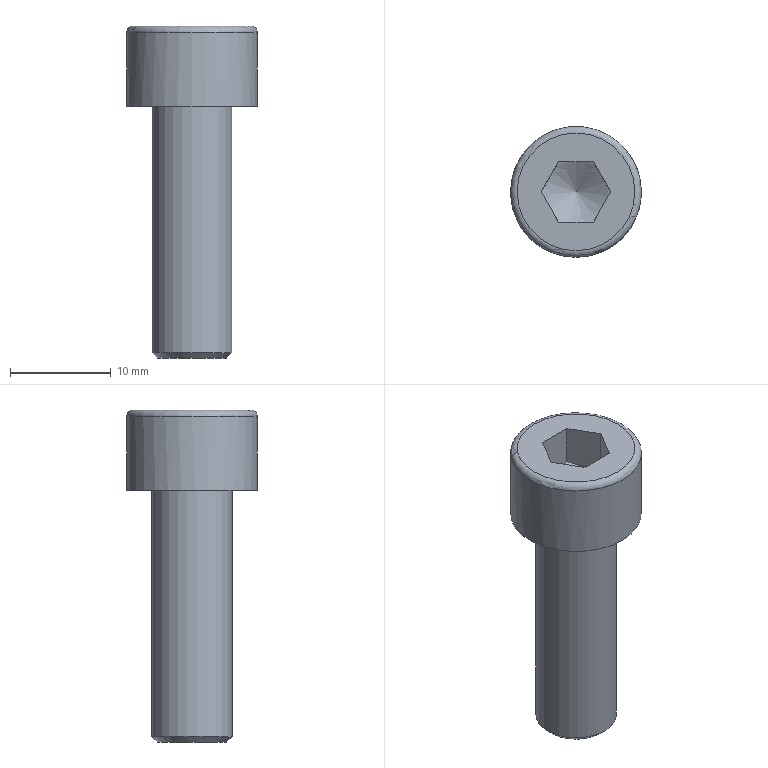Part | STEP file | 1_36 | 1 solid | 14 faces | box 13 x 13 x 33 mm | volume 2162 mm3 | plane 9 | cylinder 2 | cone 2 | torus 1 | commonest cylinder face diameters 8 x1 13 x1
STEP:
#1=CARTESIAN_POINT('',(0.,0.,0.));
#2=DIRECTION('',(0.,0.,1.));
#3=DIRECTION('',(1.,0.,0.));
#4=AXIS2_PLACEMENT_3D('',#1,#2,#3);
#5=CARTESIAN_POINT('',(0.,-6.5,-0.000000001));
#6=VERTEX_POINT('',#5);
#7=CARTESIAN_POINT('',(0.,0.,-0.000000001));
#8=DIRECTION('',(0.,0.,1.));
#9=DIRECTION('',(1.,0.,0.));
#10=AXIS2_PLACEMENT_3D('',#7,#8,#9);
#11=CIRCLE('',#10,6.5);
#12=CARTESIAN_POINT('',(0.,0.,3.675));
#13=DIRECTION('',(0.,0.,1.));
#14=DIRECTION('',(0.,-1.,0.));
#15=AXIS2_PLACEMENT_3D('',#12,#13,#14);
#16=CYLINDRICAL_SURFACE('',#15,6.5);
#17=CARTESIAN_POINT('',(-4.712,-3.675));
#18=DIRECTION('',(1.,0.));
#19=VECTOR('',#18,1.);
#20=LINE('',#17,#19);
#21=(GEOMETRIC_REPRESENTATION_CONTEXT(2)PARAMETRIC_REPRESENTATION_CONTEXT()REPRESENTATION_CONTEXT('',''));
#22=DEFINITIONAL_REPRESENTATION('',(#20),#21);
#23=PCURVE('',#16,#22);
#24=CARTESIAN_POINT('',(0.,3.25,0.));
#25=DIRECTION('',(0.,0.,-1.));
#26=DIRECTION('',(-1.,0.,0.));
#27=AXIS2_PLACEMENT_3D('',#24,#25,#26);
#28=PLANE('',#27);
#29=CARTESIAN_POINT('',(-6.5,-3.25));
#30=CARTESIAN_POINT('',(-6.5,8.008));
#31=CARTESIAN_POINT('',(3.25,2.379));
#32=CARTESIAN_POINT('',(13.,-3.25));
#33=CARTESIAN_POINT('',(3.25,-8.879));
#34=CARTESIAN_POINT('',(-6.5,-14.508));
#35=CARTESIAN_POINT('',(-6.5,-3.25));
#36=(BOUNDED_CURVE()B_SPLINE_CURVE(2,(#29,#30,#31,#32,#33,#34,#35),.UNSPECIFIED.,.T.,.F.)B_SPLINE_CURVE_WITH_KNOTS((1,2,2,2,2,1),(-2.094,0.,2.094,4.189,6.283,8.378),.UNSPECIFIED.)CURVE()GEOMETRIC_REPRESENTATION_ITEM()RATIONAL_B_SPLINE_CURVE((1.,0.5,1.,0.5,1.,0.5,1.))REPRESENTATION_ITEM(''));
#37=(GEOMETRIC_REPRESENTATION_CONTEXT(2)PARAMETRIC_REPRESENTATION_CONTEXT()REPRESENTATION_CONTEXT('',''));
#38=DEFINITIONAL_REPRESENTATION('',(#36),#37);
#39=PCURVE('',#28,#38);
#40=SURFACE_CURVE('',#11,(#23,#39),.PCURVE_S1.);
#41=EDGE_CURVE('',#6,#6,#40,.T.);
#42=ORIENTED_EDGE('',*,*,#41,.T.);
#43=CARTESIAN_POINT('',(0.,-6.5,7.35));
#44=VERTEX_POINT('',#43);
#45=CARTESIAN_POINT('',(0.,-6.5,-0.000000001));
#46=CARTESIAN_POINT('',(0.,-6.5,7.35));
#47=B_SPLINE_CURVE_WITH_KNOTS('',1,(#45,#46),.UNSPECIFIED.,.F.,.F.,(2,2),(-3.675,3.675),.PIECEWISE_BEZIER_KNOTS.);
#48=CARTESIAN_POINT('',(6.283,0.));
#49=DIRECTION('',(0.,1.));
#50=VECTOR('',#49,1.);
#51=LINE('',#48,#50);
#52=(GEOMETRIC_REPRESENTATION_CONTEXT(2)PARAMETRIC_REPRESENTATION_CONTEXT()REPRESENTATION_CONTEXT('',''));
#53=DEFINITIONAL_REPRESENTATION('',(#51),#52);
#54=PCURVE('',#16,#53);
#55=CARTESIAN_POINT('',(0.,0.));
#56=DIRECTION('',(0.,1.));
#57=VECTOR('',#56,1.);
#58=LINE('',#55,#57);
#59=(GEOMETRIC_REPRESENTATION_CONTEXT(2)PARAMETRIC_REPRESENTATION_CONTEXT()REPRESENTATION_CONTEXT('',''));
#60=DEFINITIONAL_REPRESENTATION('',(#58),#59);
#61=PCURVE('',#16,#60);
#62=SEAM_CURVE('',#47,(#54,#61),.PCURVE_S1.);
#63=EDGE_CURVE('',#6,#44,#62,.T.);
#64=ORIENTED_EDGE('',*,*,#63,.T.);
#65=CARTESIAN_POINT('',(-6.5,0.,7.35));
#66=VERTEX_POINT('',#65);
#67=CARTESIAN_POINT('',(0.,0.,7.35));
#68=DIRECTION('',(0.,0.,-1.));
#69=DIRECTION('',(0.,-1.,0.));
#70=AXIS2_PLACEMENT_3D('',#67,#68,#69);
#71=CIRCLE('',#70,6.5);
#72=CARTESIAN_POINT('',(12.566,3.675));
#73=DIRECTION('',(-1.,0.));
#74=VECTOR('',#73,1.);
#75=LINE('',#72,#74);
#76=(GEOMETRIC_REPRESENTATION_CONTEXT(2)PARAMETRIC_REPRESENTATION_CONTEXT()REPRESENTATION_CONTEXT('',''));
#77=DEFINITIONAL_REPRESENTATION('',(#75),#76);
#78=PCURVE('',#16,#77);
#79=CARTESIAN_POINT('',(0.,0.,7.35));
#80=DIRECTION('',(0.,0.,-1.));
#81=DIRECTION('',(-1.,0.,0.));
#82=AXIS2_PLACEMENT_3D('',#79,#80,#81);
#83=TOROIDAL_SURFACE('',#82,5.85,0.65);
#84=CARTESIAN_POINT('',(4.712,6.283));
#85=CARTESIAN_POINT('',(4.736,6.283));
#86=CARTESIAN_POINT('',(4.784,6.283));
#87=CARTESIAN_POINT('',(4.855,6.283));
#88=CARTESIAN_POINT('',(4.927,6.283));
#89=CARTESIAN_POINT('',(4.998,6.283));
#90=CARTESIAN_POINT('',(5.069,6.283));
#91=CARTESIAN_POINT('',(5.141,6.283));
#92=CARTESIAN_POINT('',(5.212,6.283));
#93=CARTESIAN_POINT('',(5.284,6.283));
#94=CARTESIAN_POINT('',(5.355,6.283));
#95=CARTESIAN_POINT('',(5.426,6.283));
#96=CARTESIAN_POINT('',(5.498,6.283));
#97=CARTESIAN_POINT('',(5.569,6.283));
#98=CARTESIAN_POINT('',(5.641,6.283));
#99=CARTESIAN_POINT('',(5.712,6.283));
#100=CARTESIAN_POINT('',(5.783,6.283));
#101=CARTESIAN_POINT('',(5.855,6.283));
#102=CARTESIAN_POINT('',(5.926,6.283));
#103=CARTESIAN_POINT('',(5.998,6.283));
#104=CARTESIAN_POINT('',(6.069,6.283));
#105=CARTESIAN_POINT('',(6.14,6.283));
#106=CARTESIAN_POINT('',(6.212,6.283));
#107=CARTESIAN_POINT('',(6.259,6.283));
#108=CARTESIAN_POINT('',(6.283,6.283));
#109=B_SPLINE_CURVE_WITH_KNOTS('',3,(#84,#85,#86,#87,#88,#89,#90,#91,#92,#93,#94,#95,#96,#97,#98,#99,#100,#101,#102,#103,#104,#105,#106,#107,#108),.UNSPECIFIED.,.F.,.F.,(4,1,1,1,1,1,1,1,1,1,1,1,1,1,1,1,1,1,1,1,1,1,4),(6.283,6.355,6.426,6.497,6.569,6.64,6.712,6.783,6.854,6.926,6.997,7.069,7.14,7.211,7.283,7.354,7.426,7.497,7.568,7.64,7.711,7.783,7.854),.QUASI_UNIFORM_KNOTS.);
#110=(GEOMETRIC_REPRESENTATION_CONTEXT(2)PARAMETRIC_REPRESENTATION_CONTEXT()REPRESENTATION_CONTEXT('',''));
#111=DEFINITIONAL_REPRESENTATION('',(#109),#110);
#112=PCURVE('',#83,#111);
#113=SURFACE_CURVE('',#71,(#78,#112),.PCURVE_S1.);
#114=EDGE_CURVE('',#44,#66,#113,.T.);
#115=ORIENTED_EDGE('',*,*,#114,.T.);
#116=CARTESIAN_POINT('',(6.5,0.,7.35));
#117=VERTEX_POINT('',#116);
#118=CARTESIAN_POINT('',(0.,0.,7.35));
#119=DIRECTION('',(0.,0.,1.));
#120=DIRECTION('',(1.,0.,0.));
#121=AXIS2_PLACEMENT_3D('',#118,#119,#120);
#122=CIRCLE('',#121,6.5);
#123=CARTESIAN_POINT('',(1.571,3.675));
#124=DIRECTION('',(1.,0.));
#125=VECTOR('',#124,1.);
#126=LINE('',#123,#125);
#127=(GEOMETRIC_REPRESENTATION_CONTEXT(2)PARAMETRIC_REPRESENTATION_CONTEXT()REPRESENTATION_CONTEXT('',''));
#128=DEFINITIONAL_REPRESENTATION('',(#126),#127);
#129=PCURVE('',#16,#128);
#130=CARTESIAN_POINT('',(3.142,6.283));
#131=DIRECTION('',(-1.,0.));
#132=VECTOR('',#131,1.);
#133=LINE('',#130,#132);
#134=(GEOMETRIC_REPRESENTATION_CONTEXT(2)PARAMETRIC_REPRESENTATION_CONTEXT()REPRESENTATION_CONTEXT('',''));
#135=DEFINITIONAL_REPRESENTATION('',(#133),#134);
#136=PCURVE('',#83,#135);
#137=SURFACE_CURVE('',#122,(#129,#136),.PCURVE_S1.);
#138=EDGE_CURVE('',#117,#66,#137,.T.);
#139=ORIENTED_EDGE('',*,*,#138,.F.);
#140=CARTESIAN_POINT('',(0.,0.,7.35));
#141=DIRECTION('',(0.,0.,-1.));
#142=DIRECTION('',(0.,-1.,0.));
#143=AXIS2_PLACEMENT_3D('',#140,#141,#142);
#144=CIRCLE('',#143,6.5);
#145=CARTESIAN_POINT('',(6.283,3.675));
#146=DIRECTION('',(-1.,0.));
#147=VECTOR('',#146,1.);
#148=LINE('',#145,#147);
#149=(GEOMETRIC_REPRESENTATION_CONTEXT(2)PARAMETRIC_REPRESENTATION_CONTEXT()REPRESENTATION_CONTEXT('',''));
#150=DEFINITIONAL_REPRESENTATION('',(#148),#149);
#151=PCURVE('',#16,#150);
#152=CARTESIAN_POINT('',(3.142,6.283));
#153=CARTESIAN_POINT('',(3.165,6.283));
#154=CARTESIAN_POINT('',(3.213,6.283));
#155=CARTESIAN_POINT('',(3.284,6.283));
#156=CARTESIAN_POINT('',(3.356,6.283));
#157=CARTESIAN_POINT('',(3.427,6.283));
#158=CARTESIAN_POINT('',(3.499,6.283));
#159=CARTESIAN_POINT('',(3.57,6.283));
#160=CARTESIAN_POINT('',(3.641,6.283));
#161=CARTESIAN_POINT('',(3.713,6.283));
#162=CARTESIAN_POINT('',(3.784,6.283));
#163=CARTESIAN_POINT('',(3.856,6.283));
#164=CARTESIAN_POINT('',(3.927,6.283));
#165=CARTESIAN_POINT('',(3.998,6.283));
#166=CARTESIAN_POINT('',(4.07,6.283));
#167=CARTESIAN_POINT('',(4.141,6.283));
#168=CARTESIAN_POINT('',(4.213,6.283));
#169=CARTESIAN_POINT('',(4.284,6.283));
#170=CARTESIAN_POINT('',(4.355,6.283));
#171=CARTESIAN_POINT('',(4.427,6.283));
#172=CARTESIAN_POINT('',(4.498,6.283));
#173=CARTESIAN_POINT('',(4.57,6.283));
#174=CARTESIAN_POINT('',(4.641,6.283));
#175=CARTESIAN_POINT('',(4.689,6.283));
#176=CARTESIAN_POINT('',(4.712,6.283));
#177=B_SPLINE_CURVE_WITH_KNOTS('',3,(#152,#153,#154,#155,#156,#157,#158,#159,#160,#161,#162,#163,#164,#165,#166,#167,#168,#169,#170,#171,#172,#173,#174,#175,#176),.UNSPECIFIED.,.F.,.F.,(4,1,1,1,1,1,1,1,1,1,1,1,1,1,1,1,1,1,1,1,1,1,4),(4.712,4.784,4.855,4.927,4.998,5.069,5.141,5.212,5.284,5.355,5.426,5.498,5.569,5.641,5.712,5.783,5.855,5.926,5.998,6.069,6.14,6.212,6.283),.QUASI_UNIFORM_KNOTS.);
#178=(GEOMETRIC_REPRESENTATION_CONTEXT(2)PARAMETRIC_REPRESENTATION_CONTEXT()REPRESENTATION_CONTEXT('',''));
#179=DEFINITIONAL_REPRESENTATION('',(#177),#178);
#180=PCURVE('',#83,#179);
#181=SURFACE_CURVE('',#144,(#151,#180),.PCURVE_S1.);
#182=EDGE_CURVE('',#117,#44,#181,.T.);
#183=ORIENTED_EDGE('',*,*,#182,.T.);
#184=ORIENTED_EDGE('',*,*,#63,.F.);
#185=EDGE_LOOP('',(#42,#64,#115,#139,#183,#184));
#186=FACE_BOUND('',#185,.T.);
#187=ADVANCED_FACE('',(#186),#16,.T.);
#188=ORIENTED_EDGE('',*,*,#138,.T.);
#189=CARTESIAN_POINT('',(-5.85,0.,8.));
#190=VERTEX_POINT('',#189);
#191=CARTESIAN_POINT('',(-5.85,0.,8.));
#192=CARTESIAN_POINT('',(-6.024,0.,8.));
#193=CARTESIAN_POINT('',(-6.193,0.,7.945));
#194=CARTESIAN_POINT('',(-6.339,0.,7.839));
#195=CARTESIAN_POINT('',(-6.445,0.,7.693));
#196=CARTESIAN_POINT('',(-6.5,0.,7.524));
#197=CARTESIAN_POINT('',(-6.5,0.,7.35));
#198=(BOUNDED_CURVE()B_SPLINE_CURVE(6,(#191,#192,#193,#194,#195,#196,#197),.UNSPECIFIED.,.F.,.F.)B_SPLINE_CURVE_WITH_KNOTS((7,7),(4.712,6.283),.PIECEWISE_BEZIER_KNOTS.)CURVE()GEOMETRIC_REPRESENTATION_ITEM()RATIONAL_B_SPLINE_CURVE((1.031,1.01,0.9979,0.994,0.9979,1.01,1.031))REPRESENTATION_ITEM(''));
#199=CARTESIAN_POINT('',(0.,0.));
#200=DIRECTION('',(0.,1.));
#201=VECTOR('',#200,1.);
#202=LINE('',#199,#201);
#203=(GEOMETRIC_REPRESENTATION_CONTEXT(2)PARAMETRIC_REPRESENTATION_CONTEXT()REPRESENTATION_CONTEXT('',''));
#204=DEFINITIONAL_REPRESENTATION('',(#202),#203);
#205=PCURVE('',#83,#204);
#206=CARTESIAN_POINT('',(6.283,0.));
#207=DIRECTION('',(0.,1.));
#208=VECTOR('',#207,1.);
#209=LINE('',#206,#208);
#210=(GEOMETRIC_REPRESENTATION_CONTEXT(2)PARAMETRIC_REPRESENTATION_CONTEXT()REPRESENTATION_CONTEXT('',''));
#211=DEFINITIONAL_REPRESENTATION('',(#209),#210);
#212=PCURVE('',#83,#211);
#213=SEAM_CURVE('',#198,(#205,#212),.PCURVE_S1.);
#214=EDGE_CURVE('',#190,#66,#213,.T.);
#215=ORIENTED_EDGE('',*,*,#214,.F.);
#216=CARTESIAN_POINT('',(0.,5.85,8.));
#217=VERTEX_POINT('',#216);
#218=CARTESIAN_POINT('',(0.,0.,8.));
#219=DIRECTION('',(0.,0.,-1.));
#220=DIRECTION('',(1.,0.,0.));
#221=AXIS2_PLACEMENT_3D('',#218,#219,#220);
#222=CIRCLE('',#221,5.85);
#223=CARTESIAN_POINT('',(-3.142,4.712));
#224=DIRECTION('',(1.,0.));
#225=VECTOR('',#224,1.);
#226=LINE('',#223,#225);
#227=(GEOMETRIC_REPRESENTATION_CONTEXT(2)PARAMETRIC_REPRESENTATION_CONTEXT()REPRESENTATION_CONTEXT('',''));
#228=DEFINITIONAL_REPRESENTATION('',(#226),#227);
#229=PCURVE('',#83,#228);
#230=CARTESIAN_POINT('',(0.,2.925,8.));
#231=DIRECTION('',(0.,0.,1.));
#232=DIRECTION('',(1.,0.,0.));
#233=AXIS2_PLACEMENT_3D('',#230,#231,#232);
#234=PLANE('',#233);
#235=CARTESIAN_POINT('',(5.85,-2.925));
#236=CARTESIAN_POINT('',(5.85,-13.057));
#237=CARTESIAN_POINT('',(-2.925,-7.991));
#238=CARTESIAN_POINT('',(-11.7,-2.925));
#239=CARTESIAN_POINT('',(-2.925,2.141));
#240=CARTESIAN_POINT('',(5.85,7.207));
#241=CARTESIAN_POINT('',(5.85,-2.925));
#242=(BOUNDED_CURVE()B_SPLINE_CURVE(2,(#235,#236,#237,#238,#239,#240,#241),.UNSPECIFIED.,.T.,.F.)B_SPLINE_CURVE_WITH_KNOTS((1,2,2,2,2,1),(-2.094,0.,2.094,4.189,6.283,8.378),.UNSPECIFIED.)CURVE()GEOMETRIC_REPRESENTATION_ITEM()RATIONAL_B_SPLINE_CURVE((1.,0.5,1.,0.5,1.,0.5,1.))REPRESENTATION_ITEM(''));
#243=(GEOMETRIC_REPRESENTATION_CONTEXT(2)PARAMETRIC_REPRESENTATION_CONTEXT()REPRESENTATION_CONTEXT('',''));
#244=DEFINITIONAL_REPRESENTATION('',(#242),#243);
#245=PCURVE('',#234,#244);
#246=SURFACE_CURVE('',#222,(#229,#245),.PCURVE_S1.);
#247=EDGE_CURVE('',#190,#217,#246,.T.);
#248=ORIENTED_EDGE('',*,*,#247,.T.);
#249=CARTESIAN_POINT('',(0.,0.,8.));
#250=DIRECTION('',(0.,0.,-1.));
#251=DIRECTION('',(1.,0.,0.));
#252=AXIS2_PLACEMENT_3D('',#249,#250,#251);
#253=CIRCLE('',#252,5.85);
#254=CARTESIAN_POINT('',(-3.142,4.712));
#255=DIRECTION('',(1.,0.));
#256=VECTOR('',#255,1.);
#257=LINE('',#254,#256);
#258=(GEOMETRIC_REPRESENTATION_CONTEXT(2)PARAMETRIC_REPRESENTATION_CONTEXT()REPRESENTATION_CONTEXT('',''));
#259=DEFINITIONAL_REPRESENTATION('',(#257),#258);
#260=PCURVE('',#83,#259);
#261=CARTESIAN_POINT('',(5.85,-2.925));
#262=CARTESIAN_POINT('',(5.85,-13.057));
#263=CARTESIAN_POINT('',(-2.925,-7.991));
#264=CARTESIAN_POINT('',(-11.7,-2.925));
#265=CARTESIAN_POINT('',(-2.925,2.141));
#266=CARTESIAN_POINT('',(5.85,7.207));
#267=CARTESIAN_POINT('',(5.85,-2.925));
#268=(BOUNDED_CURVE()B_SPLINE_CURVE(2,(#261,#262,#263,#264,#265,#266,#267),.UNSPECIFIED.,.T.,.F.)B_SPLINE_CURVE_WITH_KNOTS((1,2,2,2,2,1),(-2.094,0.,2.094,4.189,6.283,8.378),.UNSPECIFIED.)CURVE()GEOMETRIC_REPRESENTATION_ITEM()RATIONAL_B_SPLINE_CURVE((1.,0.5,1.,0.5,1.,0.5,1.))REPRESENTATION_ITEM(''));
#269=(GEOMETRIC_REPRESENTATION_CONTEXT(2)PARAMETRIC_REPRESENTATION_CONTEXT()REPRESENTATION_CONTEXT('',''));
#270=DEFINITIONAL_REPRESENTATION('',(#268),#269);
#271=PCURVE('',#234,#270);
#272=SURFACE_CURVE('',#253,(#260,#271),.PCURVE_S1.);
#273=EDGE_CURVE('',#217,#190,#272,.T.);
#274=ORIENTED_EDGE('',*,*,#273,.T.);
#275=ORIENTED_EDGE('',*,*,#214,.T.);
#276=ORIENTED_EDGE('',*,*,#114,.F.);
#277=ORIENTED_EDGE('',*,*,#182,.F.);
#278=EDGE_LOOP('',(#188,#215,#248,#274,#275,#276,#277));
#279=FACE_BOUND('',#278,.T.);
#280=ADVANCED_FACE('',(#279),#83,.T.);
#281=ORIENTED_EDGE('',*,*,#41,.F.);
#282=EDGE_LOOP('',(#281));
#283=FACE_BOUND('',#282,.T.);
#284=CARTESIAN_POINT('',(0.,-4.,0.));
#285=VERTEX_POINT('',#284);
#286=CARTESIAN_POINT('',(0.,0.,0.));
#287=DIRECTION('',(0.,0.,1.));
#288=DIRECTION('',(0.,1.,0.));
#289=AXIS2_PLACEMENT_3D('',#286,#287,#288);
#290=CIRCLE('',#289,4.);
#291=CARTESIAN_POINT('',(0.,0.75));
#292=CARTESIAN_POINT('',(6.928,0.75));
#293=CARTESIAN_POINT('',(3.464,-5.25));
#294=CARTESIAN_POINT('',(0.,-11.25));
#295=CARTESIAN_POINT('',(-3.464,-5.25));
#296=CARTESIAN_POINT('',(-6.928,0.75));
#297=CARTESIAN_POINT('',(0.,0.75));
#298=(BOUNDED_CURVE()B_SPLINE_CURVE(2,(#291,#292,#293,#294,#295,#296,#297),.UNSPECIFIED.,.T.,.F.)B_SPLINE_CURVE_WITH_KNOTS((1,2,2,2,2,1),(-2.094,0.,2.094,4.189,6.283,8.378),.UNSPECIFIED.)CURVE()GEOMETRIC_REPRESENTATION_ITEM()RATIONAL_B_SPLINE_CURVE((1.,0.5,1.,0.5,1.,0.5,1.))REPRESENTATION_ITEM(''));
#299=(GEOMETRIC_REPRESENTATION_CONTEXT(2)PARAMETRIC_REPRESENTATION_CONTEXT()REPRESENTATION_CONTEXT('',''));
#300=DEFINITIONAL_REPRESENTATION('',(#298),#299);
#301=PCURVE('',#28,#300);
#302=CARTESIAN_POINT('',(0.,0.,-11.729));
#303=DIRECTION('',(0.,0.,1.));
#304=DIRECTION('',(0.,-1.,0.));
#305=AXIS2_PLACEMENT_3D('',#302,#303,#304);
#306=CYLINDRICAL_SURFACE('',#305,4.);
#307=CARTESIAN_POINT('',(-3.142,11.729));
#308=DIRECTION('',(1.,0.));
#309=VECTOR('',#308,1.);
#310=LINE('',#307,#309);
#311=(GEOMETRIC_REPRESENTATION_CONTEXT(2)PARAMETRIC_REPRESENTATION_CONTEXT()REPRESENTATION_CONTEXT('',''));
#312=DEFINITIONAL_REPRESENTATION('',(#310),#311);
#313=PCURVE('',#306,#312);
#314=SURFACE_CURVE('',#290,(#301,#313),.PCURVE_S1.);
#315=EDGE_CURVE('',#285,#285,#314,.T.);
#316=ORIENTED_EDGE('',*,*,#315,.T.);
#317=EDGE_LOOP('',(#316));
#318=FACE_BOUND('',#317,.T.);
#319=ADVANCED_FACE('',(#283,#318),#28,.T.);
#320=ORIENTED_EDGE('',*,*,#273,.F.);
#321=ORIENTED_EDGE('',*,*,#247,.F.);
#322=EDGE_LOOP('',(#320,#321));
#323=FACE_BOUND('',#322,.T.);
#324=CARTESIAN_POINT('',(-1.732,-3.,8.));
#325=VERTEX_POINT('',#324);
#326=CARTESIAN_POINT('',(-3.464,0.,8.));
#327=VERTEX_POINT('',#326);
#328=CARTESIAN_POINT('',(-1.732,-3.,8.));
#329=DIRECTION('',(-0.5,0.866,0.));
#330=VECTOR('',#329,1.);
#331=LINE('',#328,#330);
#332=CARTESIAN_POINT('',(-1.732,-5.925));
#333=DIRECTION('',(-0.5,0.866));
#334=VECTOR('',#333,1.);
#335=LINE('',#332,#334);
#336=(GEOMETRIC_REPRESENTATION_CONTEXT(2)PARAMETRIC_REPRESENTATION_CONTEXT()REPRESENTATION_CONTEXT('',''));
#337=DEFINITIONAL_REPRESENTATION('',(#335),#336);
#338=PCURVE('',#234,#337);
#339=CARTESIAN_POINT('',(-3.464,0.,8.));
#340=DIRECTION('',(-0.866,-0.5,0.));
#341=DIRECTION('',(0.,0.,1.));
#342=AXIS2_PLACEMENT_3D('',#339,#340,#341);
#343=PLANE('',#342);
#344=CARTESIAN_POINT('',(0.,-3.464));
#345=DIRECTION('',(0.,1.));
#346=VECTOR('',#345,1.);
#347=LINE('',#344,#346);
#348=(GEOMETRIC_REPRESENTATION_CONTEXT(2)PARAMETRIC_REPRESENTATION_CONTEXT()REPRESENTATION_CONTEXT('',''));
#349=DEFINITIONAL_REPRESENTATION('',(#347),#348);
#350=PCURVE('',#343,#349);
#351=SURFACE_CURVE('',#331,(#338,#350),.PCURVE_S1.);
#352=EDGE_CURVE('',#325,#327,#351,.T.);
#353=ORIENTED_EDGE('',*,*,#352,.T.);
#354=CARTESIAN_POINT('',(-1.732,3.,8.));
#355=VERTEX_POINT('',#354);
#356=CARTESIAN_POINT('',(-3.464,0.,8.));
#357=DIRECTION('',(0.5,0.866,0.));
#358=VECTOR('',#357,1.);
#359=LINE('',#356,#358);
#360=CARTESIAN_POINT('',(-3.464,-2.925));
#361=DIRECTION('',(0.5,0.866));
#362=VECTOR('',#361,1.);
#363=LINE('',#360,#362);
#364=(GEOMETRIC_REPRESENTATION_CONTEXT(2)PARAMETRIC_REPRESENTATION_CONTEXT()REPRESENTATION_CONTEXT('',''));
#365=DEFINITIONAL_REPRESENTATION('',(#363),#364);
#366=PCURVE('',#234,#365);
#367=CARTESIAN_POINT('',(-1.732,3.,8.));
#368=DIRECTION('',(-0.866,0.5,0.));
#369=DIRECTION('',(0.,0.,1.));
#370=AXIS2_PLACEMENT_3D('',#367,#368,#369);
#371=PLANE('',#370);
#372=CARTESIAN_POINT('',(0.,-3.464));
#373=DIRECTION('',(0.,1.));
#374=VECTOR('',#373,1.);
#375=LINE('',#372,#374);
#376=(GEOMETRIC_REPRESENTATION_CONTEXT(2)PARAMETRIC_REPRESENTATION_CONTEXT()REPRESENTATION_CONTEXT('',''));
#377=DEFINITIONAL_REPRESENTATION('',(#375),#376);
#378=PCURVE('',#371,#377);
#379=SURFACE_CURVE('',#359,(#366,#378),.PCURVE_S1.);
#380=EDGE_CURVE('',#327,#355,#379,.T.);
#381=ORIENTED_EDGE('',*,*,#380,.T.);
#382=CARTESIAN_POINT('',(1.732,3.,8.));
#383=VERTEX_POINT('',#382);
#384=CARTESIAN_POINT('',(-1.732,3.,8.));
#385=DIRECTION('',(1.,0.,0.));
#386=VECTOR('',#385,1.);
#387=LINE('',#384,#386);
#388=CARTESIAN_POINT('',(-1.732,0.075));
#389=DIRECTION('',(1.,0.));
#390=VECTOR('',#389,1.);
#391=LINE('',#388,#390);
#392=(GEOMETRIC_REPRESENTATION_CONTEXT(2)PARAMETRIC_REPRESENTATION_CONTEXT()REPRESENTATION_CONTEXT('',''));
#393=DEFINITIONAL_REPRESENTATION('',(#391),#392);
#394=PCURVE('',#234,#393);
#395=CARTESIAN_POINT('',(1.732,3.,8.));
#396=DIRECTION('',(0.,1.,0.));
#397=DIRECTION('',(0.,0.,1.));
#398=AXIS2_PLACEMENT_3D('',#395,#396,#397);
#399=PLANE('',#398);
#400=CARTESIAN_POINT('',(0.,-3.464));
#401=DIRECTION('',(0.,1.));
#402=VECTOR('',#401,1.);
#403=LINE('',#400,#402);
#404=(GEOMETRIC_REPRESENTATION_CONTEXT(2)PARAMETRIC_REPRESENTATION_CONTEXT()REPRESENTATION_CONTEXT('',''));
#405=DEFINITIONAL_REPRESENTATION('',(#403),#404);
#406=PCURVE('',#399,#405);
#407=SURFACE_CURVE('',#387,(#394,#406),.PCURVE_S1.);
#408=EDGE_CURVE('',#355,#383,#407,.T.);
#409=ORIENTED_EDGE('',*,*,#408,.T.);
#410=CARTESIAN_POINT('',(3.464,0.,8.));
#411=VERTEX_POINT('',#410);
#412=CARTESIAN_POINT('',(1.732,3.,8.));
#413=DIRECTION('',(0.5,-0.866,0.));
#414=VECTOR('',#413,1.);
#415=LINE('',#412,#414);
#416=CARTESIAN_POINT('',(1.732,0.075));
#417=DIRECTION('',(0.5,-0.866));
#418=VECTOR('',#417,1.);
#419=LINE('',#416,#418);
#420=(GEOMETRIC_REPRESENTATION_CONTEXT(2)PARAMETRIC_REPRESENTATION_CONTEXT()REPRESENTATION_CONTEXT('',''));
#421=DEFINITIONAL_REPRESENTATION('',(#419),#420);
#422=PCURVE('',#234,#421);
#423=CARTESIAN_POINT('',(3.464,0.,8.));
#424=DIRECTION('',(0.866,0.5,0.));
#425=DIRECTION('',(0.,0.,-1.));
#426=AXIS2_PLACEMENT_3D('',#423,#424,#425);
#427=PLANE('',#426);
#428=CARTESIAN_POINT('',(0.,3.464));
#429=DIRECTION('',(0.,-1.));
#430=VECTOR('',#429,1.);
#431=LINE('',#428,#430);
#432=(GEOMETRIC_REPRESENTATION_CONTEXT(2)PARAMETRIC_REPRESENTATION_CONTEXT()REPRESENTATION_CONTEXT('',''));
#433=DEFINITIONAL_REPRESENTATION('',(#431),#432);
#434=PCURVE('',#427,#433);
#435=SURFACE_CURVE('',#415,(#422,#434),.PCURVE_S1.);
#436=EDGE_CURVE('',#383,#411,#435,.T.);
#437=ORIENTED_EDGE('',*,*,#436,.T.);
#438=CARTESIAN_POINT('',(1.732,-3.,8.));
#439=VERTEX_POINT('',#438);
#440=CARTESIAN_POINT('',(3.464,0.,8.));
#441=DIRECTION('',(-0.5,-0.866,0.));
#442=VECTOR('',#441,1.);
#443=LINE('',#440,#442);
#444=CARTESIAN_POINT('',(3.464,-2.925));
#445=DIRECTION('',(-0.5,-0.866));
#446=VECTOR('',#445,1.);
#447=LINE('',#444,#446);
#448=(GEOMETRIC_REPRESENTATION_CONTEXT(2)PARAMETRIC_REPRESENTATION_CONTEXT()REPRESENTATION_CONTEXT('',''));
#449=DEFINITIONAL_REPRESENTATION('',(#447),#448);
#450=PCURVE('',#234,#449);
#451=CARTESIAN_POINT('',(1.732,-3.,8.));
#452=DIRECTION('',(0.866,-0.5,0.));
#453=DIRECTION('',(0.,0.,-1.));
#454=AXIS2_PLACEMENT_3D('',#451,#452,#453);
#455=PLANE('',#454);
#456=CARTESIAN_POINT('',(0.,3.464));
#457=DIRECTION('',(0.,-1.));
#458=VECTOR('',#457,1.);
#459=LINE('',#456,#458);
#460=(GEOMETRIC_REPRESENTATION_CONTEXT(2)PARAMETRIC_REPRESENTATION_CONTEXT()REPRESENTATION_CONTEXT('',''));
#461=DEFINITIONAL_REPRESENTATION('',(#459),#460);
#462=PCURVE('',#455,#461);
#463=SURFACE_CURVE('',#443,(#450,#462),.PCURVE_S1.);
#464=EDGE_CURVE('',#411,#439,#463,.T.);
#465=ORIENTED_EDGE('',*,*,#464,.T.);
#466=CARTESIAN_POINT('',(1.732,-3.,8.));
#467=DIRECTION('',(-1.,0.,0.));
#468=VECTOR('',#467,1.);
#469=LINE('',#466,#468);
#470=CARTESIAN_POINT('',(1.732,-5.925));
#471=DIRECTION('',(-1.,0.));
#472=VECTOR('',#471,1.);
#473=LINE('',#470,#472);
#474=(GEOMETRIC_REPRESENTATION_CONTEXT(2)PARAMETRIC_REPRESENTATION_CONTEXT()REPRESENTATION_CONTEXT('',''));
#475=DEFINITIONAL_REPRESENTATION('',(#473),#474);
#476=PCURVE('',#234,#475);
#477=CARTESIAN_POINT('',(-1.732,-3.,8.));
#478=DIRECTION('',(0.,-1.,0.));
#479=DIRECTION('',(0.,0.,-1.));
#480=AXIS2_PLACEMENT_3D('',#477,#478,#479);
#481=PLANE('',#480);
#482=CARTESIAN_POINT('',(0.,3.464));
#483=DIRECTION('',(0.,-1.));
#484=VECTOR('',#483,1.);
#485=LINE('',#482,#484);
#486=(GEOMETRIC_REPRESENTATION_CONTEXT(2)PARAMETRIC_REPRESENTATION_CONTEXT()REPRESENTATION_CONTEXT('',''));
#487=DEFINITIONAL_REPRESENTATION('',(#485),#486);
#488=PCURVE('',#481,#487);
#489=SURFACE_CURVE('',#469,(#476,#488),.PCURVE_S1.);
#490=EDGE_CURVE('',#439,#325,#489,.T.);
#491=ORIENTED_EDGE('',*,*,#490,.T.);
#492=EDGE_LOOP('',(#353,#381,#409,#437,#465,#491));
#493=FACE_BOUND('',#492,.T.);
#494=ADVANCED_FACE('',(#323,#493),#234,.T.);
#495=CARTESIAN_POINT('',(0.,-4.,-24.459));
#496=VERTEX_POINT('',#495);
#497=CARTESIAN_POINT('',(0.,0.,-24.459));
#498=DIRECTION('',(0.,0.,1.));
#499=DIRECTION('',(1.,0.,0.));
#500=AXIS2_PLACEMENT_3D('',#497,#498,#499);
#501=CIRCLE('',#500,4.);
#502=CARTESIAN_POINT('',(-4.712,-12.729));
#503=DIRECTION('',(1.,0.));
#504=VECTOR('',#503,1.);
#505=LINE('',#502,#504);
#506=(GEOMETRIC_REPRESENTATION_CONTEXT(2)PARAMETRIC_REPRESENTATION_CONTEXT()REPRESENTATION_CONTEXT('',''));
#507=DEFINITIONAL_REPRESENTATION('',(#505),#506);
#508=PCURVE('',#306,#507);
#509=CARTESIAN_POINT('',(0.,0.,-24.729));
#510=DIRECTION('',(0.,0.,1.));
#511=DIRECTION('',(0.,-1.,0.));
#512=AXIS2_PLACEMENT_3D('',#509,#510,#511);
#513=CONICAL_SURFACE('',#512,3.729,0.7854);
#514=CARTESIAN_POINT('',(-4.712,0.2706));
#515=DIRECTION('',(1.,0.));
#516=VECTOR('',#515,1.);
#517=LINE('',#514,#516);
#518=(GEOMETRIC_REPRESENTATION_CONTEXT(2)PARAMETRIC_REPRESENTATION_CONTEXT()REPRESENTATION_CONTEXT('',''));
#519=DEFINITIONAL_REPRESENTATION('',(#517),#518);
#520=PCURVE('',#513,#519);
#521=SURFACE_CURVE('',#501,(#508,#520),.PCURVE_S1.);
#522=EDGE_CURVE('',#496,#496,#521,.T.);
#523=ORIENTED_EDGE('',*,*,#522,.T.);
#524=CARTESIAN_POINT('',(0.,-4.,-24.459));
#525=CARTESIAN_POINT('',(0.,-4.,0.));
#526=B_SPLINE_CURVE_WITH_KNOTS('',1,(#524,#525),.UNSPECIFIED.,.F.,.F.,(2,2),(-12.729,11.729),.PIECEWISE_BEZIER_KNOTS.);
#527=CARTESIAN_POINT('',(6.283,0.));
#528=DIRECTION('',(0.,1.));
#529=VECTOR('',#528,1.);
#530=LINE('',#527,#529);
#531=(GEOMETRIC_REPRESENTATION_CONTEXT(2)PARAMETRIC_REPRESENTATION_CONTEXT()REPRESENTATION_CONTEXT('',''));
#532=DEFINITIONAL_REPRESENTATION('',(#530),#531);
#533=PCURVE('',#306,#532);
#534=CARTESIAN_POINT('',(0.,0.));
#535=DIRECTION('',(0.,1.));
#536=VECTOR('',#535,1.);
#537=LINE('',#534,#536);
#538=(GEOMETRIC_REPRESENTATION_CONTEXT(2)PARAMETRIC_REPRESENTATION_CONTEXT()REPRESENTATION_CONTEXT('',''));
#539=DEFINITIONAL_REPRESENTATION('',(#537),#538);
#540=PCURVE('',#306,#539);
#541=SEAM_CURVE('',#526,(#533,#540),.PCURVE_S1.);
#542=EDGE_CURVE('',#496,#285,#541,.T.);
#543=ORIENTED_EDGE('',*,*,#542,.T.);
#544=ORIENTED_EDGE('',*,*,#315,.F.);
#545=ORIENTED_EDGE('',*,*,#542,.F.);
#546=EDGE_LOOP('',(#523,#543,#544,#545));
#547=FACE_BOUND('',#546,.T.);
#548=ADVANCED_FACE('',(#547),#306,.T.);
#549=CARTESIAN_POINT('',(-1.732,-3.,4.));
#550=VERTEX_POINT('',#549);
#551=CARTESIAN_POINT('',(-3.464,0.,4.));
#552=VERTEX_POINT('',#551);
#553=CARTESIAN_POINT('',(3.276,-11.673,9.));
#554=CARTESIAN_POINT('',(-2.598,-1.5,2.429));
#555=CARTESIAN_POINT('',(-8.472,8.673,9.));
#556=(BOUNDED_CURVE()B_SPLINE_CURVE(2,(#553,#554,#555),.UNSPECIFIED.,.F.,.F.)B_SPLINE_CURVE_WITH_KNOTS((3,3),(0.,2.575),.PIECEWISE_BEZIER_KNOTS.)CURVE()GEOMETRIC_REPRESENTATION_ITEM()RATIONAL_B_SPLINE_CURVE((1.,4.041,1.))REPRESENTATION_ITEM(''));
#557=CARTESIAN_POINT('',(1.,-13.479));
#558=CARTESIAN_POINT('',(-5.571,-1.732));
#559=CARTESIAN_POINT('',(1.,10.015));
#560=(BOUNDED_CURVE()B_SPLINE_CURVE(2,(#557,#558,#559),.UNSPECIFIED.,.F.,.F.)B_SPLINE_CURVE_WITH_KNOTS((3,3),(0.,2.575),.PIECEWISE_BEZIER_KNOTS.)CURVE()GEOMETRIC_REPRESENTATION_ITEM()RATIONAL_B_SPLINE_CURVE((1.,4.041,1.))REPRESENTATION_ITEM(''));
#561=(GEOMETRIC_REPRESENTATION_CONTEXT(2)PARAMETRIC_REPRESENTATION_CONTEXT()REPRESENTATION_CONTEXT('',''));
#562=DEFINITIONAL_REPRESENTATION('',(#560),#561);
#563=PCURVE('',#343,#562);
#564=CARTESIAN_POINT('',(0.,0.,3.));
#565=DIRECTION('',(0.,0.,1.));
#566=DIRECTION('',(0.,1.,0.));
#567=AXIS2_PLACEMENT_3D('',#564,#565,#566);
#568=CONICAL_SURFACE('',#567,1.732,1.047);
#569=CARTESIAN_POINT('',(2.618,1.));
#570=CARTESIAN_POINT('',(2.603,0.9825));
#571=CARTESIAN_POINT('',(2.572,0.9496));
#572=CARTESIAN_POINT('',(2.526,0.906));
#573=CARTESIAN_POINT('',(2.479,0.8679));
#574=CARTESIAN_POINT('',(2.432,0.835));
#575=CARTESIAN_POINT('',(2.385,0.8069));
#576=CARTESIAN_POINT('',(2.337,0.7835));
#577=CARTESIAN_POINT('',(2.289,0.7645));
#578=CARTESIAN_POINT('',(2.24,0.7499));
#579=CARTESIAN_POINT('',(2.192,0.7396));
#580=CARTESIAN_POINT('',(2.143,0.7334));
#581=CARTESIAN_POINT('',(2.094,0.7314));
#582=CARTESIAN_POINT('',(2.046,0.7334));
#583=CARTESIAN_POINT('',(1.997,0.7396));
#584=CARTESIAN_POINT('',(1.948,0.7499));
#585=CARTESIAN_POINT('',(1.9,0.7645));
#586=CARTESIAN_POINT('',(1.852,0.7835));
#587=CARTESIAN_POINT('',(1.804,0.8069));
#588=CARTESIAN_POINT('',(1.757,0.835));
#589=CARTESIAN_POINT('',(1.709,0.8679));
#590=CARTESIAN_POINT('',(1.663,0.906));
#591=CARTESIAN_POINT('',(1.616,0.9496));
#592=CARTESIAN_POINT('',(1.586,0.9825));
#593=CARTESIAN_POINT('',(1.571,1.));
#594=B_SPLINE_CURVE_WITH_KNOTS('',3,(#569,#570,#571,#572,#573,#574,#575,#576,#577,#578,#579,#580,#581,#582,#583,#584,#585,#586,#587,#588,#589,#590,#591,#592,#593),.UNSPECIFIED.,.F.,.F.,(4,1,1,1,1,1,1,1,1,1,1,1,1,1,1,1,1,1,1,1,1,1,4),(0.8433,0.8837,0.9241,0.9644,1.005,1.045,1.086,1.126,1.166,1.207,1.247,1.287,1.328,1.368,1.409,1.449,1.489,1.53,1.57,1.61,1.651,1.691,1.732),.QUASI_UNIFORM_KNOTS.);
#595=(GEOMETRIC_REPRESENTATION_CONTEXT(2)PARAMETRIC_REPRESENTATION_CONTEXT()REPRESENTATION_CONTEXT('',''));
#596=DEFINITIONAL_REPRESENTATION('',(#594),#595);
#597=PCURVE('',#568,#596);
#598=SURFACE_CURVE('',#556,(#563,#597),.PCURVE_S1.);
#599=EDGE_CURVE('',#550,#552,#598,.T.);
#600=ORIENTED_EDGE('',*,*,#599,.T.);
#601=CARTESIAN_POINT('',(-3.464,0.,8.));
#602=DIRECTION('',(0.,0.,-1.));
#603=VECTOR('',#602,1.);
#604=LINE('',#601,#603);
#605=CARTESIAN_POINT('',(0.,0.));
#606=DIRECTION('',(-1.,0.));
#607=VECTOR('',#606,1.);
#608=LINE('',#605,#607);
#609=(GEOMETRIC_REPRESENTATION_CONTEXT(2)PARAMETRIC_REPRESENTATION_CONTEXT()REPRESENTATION_CONTEXT('',''));
#610=DEFINITIONAL_REPRESENTATION('',(#608),#609);
#611=PCURVE('',#343,#610);
#612=CARTESIAN_POINT('',(0.,-3.464));
#613=DIRECTION('',(-1.,0.));
#614=VECTOR('',#613,1.);
#615=LINE('',#612,#614);
#616=(GEOMETRIC_REPRESENTATION_CONTEXT(2)PARAMETRIC_REPRESENTATION_CONTEXT()REPRESENTATION_CONTEXT('',''));
#617=DEFINITIONAL_REPRESENTATION('',(#615),#616);
#618=PCURVE('',#371,#617);
#619=SURFACE_CURVE('',#604,(#611,#618),.PCURVE_S1.);
#620=EDGE_CURVE('',#327,#552,#619,.T.);
#621=ORIENTED_EDGE('',*,*,#620,.F.);
#622=ORIENTED_EDGE('',*,*,#352,.F.);
#623=CARTESIAN_POINT('',(-1.732,-3.,8.));
#624=DIRECTION('',(0.,0.,-1.));
#625=VECTOR('',#624,1.);
#626=LINE('',#623,#625);
#627=CARTESIAN_POINT('',(0.,-3.464));
#628=DIRECTION('',(-1.,0.));
#629=VECTOR('',#628,1.);
#630=LINE('',#627,#629);
#631=(GEOMETRIC_REPRESENTATION_CONTEXT(2)PARAMETRIC_REPRESENTATION_CONTEXT()REPRESENTATION_CONTEXT('',''));
#632=DEFINITIONAL_REPRESENTATION('',(#630),#631);
#633=PCURVE('',#343,#632);
#634=CARTESIAN_POINT('',(0.,0.));
#635=DIRECTION('',(1.,0.));
#636=VECTOR('',#635,1.);
#637=LINE('',#634,#636);
#638=(GEOMETRIC_REPRESENTATION_CONTEXT(2)PARAMETRIC_REPRESENTATION_CONTEXT()REPRESENTATION_CONTEXT('',''));
#639=DEFINITIONAL_REPRESENTATION('',(#637),#638);
#640=PCURVE('',#481,#639);
#641=SURFACE_CURVE('',#626,(#633,#640),.PCURVE_S1.);
#642=EDGE_CURVE('',#325,#550,#641,.T.);
#643=ORIENTED_EDGE('',*,*,#642,.T.);
#644=EDGE_LOOP('',(#600,#621,#622,#643));
#645=FACE_BOUND('',#644,.T.);
#646=ADVANCED_FACE('',(#645),#343,.F.);
#647=CARTESIAN_POINT('',(-1.732,3.,4.));
#648=VERTEX_POINT('',#647);
#649=CARTESIAN_POINT('',(-8.472,-8.673,9.));
#650=CARTESIAN_POINT('',(-2.598,1.5,2.429));
#651=CARTESIAN_POINT('',(3.276,11.673,9.));
#652=(BOUNDED_CURVE()B_SPLINE_CURVE(2,(#649,#650,#651),.UNSPECIFIED.,.F.,.F.)B_SPLINE_CURVE_WITH_KNOTS((3,3),(0.,2.575),.PIECEWISE_BEZIER_KNOTS.)CURVE()GEOMETRIC_REPRESENTATION_ITEM()RATIONAL_B_SPLINE_CURVE((1.,4.041,1.))REPRESENTATION_ITEM(''));
#653=CARTESIAN_POINT('',(1.,-13.479));
#654=CARTESIAN_POINT('',(-5.571,-1.732));
#655=CARTESIAN_POINT('',(1.,10.015));
#656=(BOUNDED_CURVE()B_SPLINE_CURVE(2,(#653,#654,#655),.UNSPECIFIED.,.F.,.F.)B_SPLINE_CURVE_WITH_KNOTS((3,3),(0.,2.575),.PIECEWISE_BEZIER_KNOTS.)CURVE()GEOMETRIC_REPRESENTATION_ITEM()RATIONAL_B_SPLINE_CURVE((1.,4.041,1.))REPRESENTATION_ITEM(''));
#657=(GEOMETRIC_REPRESENTATION_CONTEXT(2)PARAMETRIC_REPRESENTATION_CONTEXT()REPRESENTATION_CONTEXT('',''));
#658=DEFINITIONAL_REPRESENTATION('',(#656),#657);
#659=PCURVE('',#371,#658);
#660=CARTESIAN_POINT('',(1.571,1.));
#661=CARTESIAN_POINT('',(1.556,0.9825));
#662=CARTESIAN_POINT('',(1.525,0.9496));
#663=CARTESIAN_POINT('',(1.479,0.906));
#664=CARTESIAN_POINT('',(1.432,0.8679));
#665=CARTESIAN_POINT('',(1.385,0.835));
#666=CARTESIAN_POINT('',(1.338,0.8069));
#667=CARTESIAN_POINT('',(1.29,0.7835));
#668=CARTESIAN_POINT('',(1.241,0.7645));
#669=CARTESIAN_POINT('',(1.193,0.7499));
#670=CARTESIAN_POINT('',(1.145,0.7396));
#671=CARTESIAN_POINT('',(1.096,0.7334));
#672=CARTESIAN_POINT('',(1.047,0.7314));
#673=CARTESIAN_POINT('',(0.9985,0.7334));
#674=CARTESIAN_POINT('',(0.9498,0.7396));
#675=CARTESIAN_POINT('',(0.9013,0.7499));
#676=CARTESIAN_POINT('',(0.8529,0.7645));
#677=CARTESIAN_POINT('',(0.8048,0.7835));
#678=CARTESIAN_POINT('',(0.7569,0.8069));
#679=CARTESIAN_POINT('',(0.7094,0.835));
#680=CARTESIAN_POINT('',(0.6622,0.8679));
#681=CARTESIAN_POINT('',(0.6155,0.906));
#682=CARTESIAN_POINT('',(0.5692,0.9496));
#683=CARTESIAN_POINT('',(0.5388,0.9825));
#684=CARTESIAN_POINT('',(0.5236,1.));
#685=B_SPLINE_CURVE_WITH_KNOTS('',3,(#660,#661,#662,#663,#664,#665,#666,#667,#668,#669,#670,#671,#672,#673,#674,#675,#676,#677,#678,#679,#680,#681,#682,#683,#684),.UNSPECIFIED.,.F.,.F.,(4,1,1,1,1,1,1,1,1,1,1,1,1,1,1,1,1,1,1,1,1,1,4),(0.8433,0.8837,0.9241,0.9644,1.005,1.045,1.086,1.126,1.166,1.207,1.247,1.287,1.328,1.368,1.409,1.449,1.489,1.53,1.57,1.61,1.651,1.691,1.732),.QUASI_UNIFORM_KNOTS.);
#686=(GEOMETRIC_REPRESENTATION_CONTEXT(2)PARAMETRIC_REPRESENTATION_CONTEXT()REPRESENTATION_CONTEXT('',''));
#687=DEFINITIONAL_REPRESENTATION('',(#685),#686);
#688=PCURVE('',#568,#687);
#689=SURFACE_CURVE('',#652,(#659,#688),.PCURVE_S1.);
#690=EDGE_CURVE('',#552,#648,#689,.T.);
#691=ORIENTED_EDGE('',*,*,#690,.T.);
#692=CARTESIAN_POINT('',(-1.732,3.,8.));
#693=DIRECTION('',(0.,0.,-1.));
#694=VECTOR('',#693,1.);
#695=LINE('',#692,#694);
#696=CARTESIAN_POINT('',(0.,0.));
#697=DIRECTION('',(-1.,0.));
#698=VECTOR('',#697,1.);
#699=LINE('',#696,#698);
#700=(GEOMETRIC_REPRESENTATION_CONTEXT(2)PARAMETRIC_REPRESENTATION_CONTEXT()REPRESENTATION_CONTEXT('',''));
#701=DEFINITIONAL_REPRESENTATION('',(#699),#700);
#702=PCURVE('',#371,#701);
#703=CARTESIAN_POINT('',(0.,-3.464));
#704=DIRECTION('',(-1.,0.));
#705=VECTOR('',#704,1.);
#706=LINE('',#703,#705);
#707=(GEOMETRIC_REPRESENTATION_CONTEXT(2)PARAMETRIC_REPRESENTATION_CONTEXT()REPRESENTATION_CONTEXT('',''));
#708=DEFINITIONAL_REPRESENTATION('',(#706),#707);
#709=PCURVE('',#399,#708);
#710=SURFACE_CURVE('',#695,(#702,#709),.PCURVE_S1.);
#711=EDGE_CURVE('',#355,#648,#710,.T.);
#712=ORIENTED_EDGE('',*,*,#711,.F.);
#713=ORIENTED_EDGE('',*,*,#380,.F.);
#714=ORIENTED_EDGE('',*,*,#620,.T.);
#715=EDGE_LOOP('',(#691,#712,#713,#714));
#716=FACE_BOUND('',#715,.T.);
#717=ADVANCED_FACE('',(#716),#371,.F.);
#718=CARTESIAN_POINT('',(0.,3.,3.732));
#719=VERTEX_POINT('',#718);
#720=CARTESIAN_POINT('',(-1.732,3.,4.));
#721=CARTESIAN_POINT('',(-1.366,3.,3.894));
#722=CARTESIAN_POINT('',(-1.013,3.,3.813));
#723=CARTESIAN_POINT('',(-0.6709,3.,3.759));
#724=CARTESIAN_POINT('',(-0.3355,3.,3.732));
#725=CARTESIAN_POINT('',(0.,3.,3.732));
#726=B_SPLINE_CURVE_WITH_KNOTS('',5,(#720,#721,#722,#723,#724,#725),.UNSPECIFIED.,.F.,.F.,(6,6),(0.,2.52),.PIECEWISE_BEZIER_KNOTS.);
#727=CARTESIAN_POINT('',(-4.,-3.464));
#728=CARTESIAN_POINT('',(-4.106,-3.098));
#729=CARTESIAN_POINT('',(-4.187,-2.745));
#730=CARTESIAN_POINT('',(-4.241,-2.403));
#731=CARTESIAN_POINT('',(-4.268,-2.068));
#732=CARTESIAN_POINT('',(-4.268,-1.732));
#733=B_SPLINE_CURVE_WITH_KNOTS('',5,(#727,#728,#729,#730,#731,#732),.UNSPECIFIED.,.F.,.F.,(6,6),(0.,2.52),.PIECEWISE_BEZIER_KNOTS.);
#734=(GEOMETRIC_REPRESENTATION_CONTEXT(2)PARAMETRIC_REPRESENTATION_CONTEXT()REPRESENTATION_CONTEXT('',''));
#735=DEFINITIONAL_REPRESENTATION('',(#733),#734);
#736=PCURVE('',#399,#735);
#737=CARTESIAN_POINT('',(0.5236,1.));
#738=CARTESIAN_POINT('',(0.5167,0.992));
#739=CARTESIAN_POINT('',(0.5027,0.9763));
#740=CARTESIAN_POINT('',(0.4813,0.9538));
#741=CARTESIAN_POINT('',(0.4596,0.9324));
#742=CARTESIAN_POINT('',(0.4376,0.912));
#743=CARTESIAN_POINT('',(0.4152,0.8927));
#744=CARTESIAN_POINT('',(0.3926,0.8744));
#745=CARTESIAN_POINT('',(0.3696,0.8573));
#746=CARTESIAN_POINT('',(0.3463,0.8412));
#747=CARTESIAN_POINT('',(0.3228,0.8262));
#748=CARTESIAN_POINT('',(0.299,0.8122));
#749=CARTESIAN_POINT('',(0.2749,0.7994));
#750=CARTESIAN_POINT('',(0.2507,0.7877));
#751=CARTESIAN_POINT('',(0.2262,0.7771));
#752=CARTESIAN_POINT('',(0.2015,0.7676));
#753=CARTESIAN_POINT('',(0.1767,0.7593));
#754=CARTESIAN_POINT('',(0.1517,0.752));
#755=CARTESIAN_POINT('',(0.1266,0.7458));
#756=CARTESIAN_POINT('',(0.1014,0.7408));
#757=CARTESIAN_POINT('',(0.07616,0.7369));
#758=CARTESIAN_POINT('',(0.05081,0.7341));
#759=CARTESIAN_POINT('',(0.02541,0.7324));
#760=CARTESIAN_POINT('',(0.008472,0.7321));
#761=CARTESIAN_POINT('',(0.,0.7321));
#762=B_SPLINE_CURVE_WITH_KNOTS('',3,(#737,#738,#739,#740,#741,#742,#743,#744,#745,#746,#747,#748,#749,#750,#751,#752,#753,#754,#755,#756,#757,#758,#759,#760,#761),.UNSPECIFIED.,.F.,.F.,(4,1,1,1,1,1,1,1,1,1,1,1,1,1,1,1,1,1,1,1,1,1,4),(0.,0.1146,0.2291,0.3437,0.4582,0.5728,0.6873,0.8019,0.9164,1.031,1.146,1.26,1.375,1.489,1.604,1.718,1.833,1.947,2.062,2.177,2.291,2.406,2.52),.QUASI_UNIFORM_KNOTS.);
#763=(GEOMETRIC_REPRESENTATION_CONTEXT(2)PARAMETRIC_REPRESENTATION_CONTEXT()REPRESENTATION_CONTEXT('',''));
#764=DEFINITIONAL_REPRESENTATION('',(#762),#763);
#765=PCURVE('',#568,#764);
#766=SURFACE_CURVE('',#726,(#736,#765),.PCURVE_S1.);
#767=EDGE_CURVE('',#648,#719,#766,.T.);
#768=ORIENTED_EDGE('',*,*,#767,.T.);
#769=CARTESIAN_POINT('',(1.732,3.,4.));
#770=VERTEX_POINT('',#769);
#771=CARTESIAN_POINT('',(0.,3.,3.732));
#772=CARTESIAN_POINT('',(0.3355,3.,3.732));
#773=CARTESIAN_POINT('',(0.6709,3.,3.759));
#774=CARTESIAN_POINT('',(1.013,3.,3.813));
#775=CARTESIAN_POINT('',(1.366,3.,3.894));
#776=CARTESIAN_POINT('',(1.732,3.,4.));
#777=B_SPLINE_CURVE_WITH_KNOTS('',5,(#771,#772,#773,#774,#775,#776),.UNSPECIFIED.,.F.,.F.,(6,6),(0.,2.52),.PIECEWISE_BEZIER_KNOTS.);
#778=CARTESIAN_POINT('',(-4.268,-1.732));
#779=CARTESIAN_POINT('',(-4.268,-1.397));
#780=CARTESIAN_POINT('',(-4.241,-1.061));
#781=CARTESIAN_POINT('',(-4.187,-0.7194));
#782=CARTESIAN_POINT('',(-4.106,-0.3661));
#783=CARTESIAN_POINT('',(-4.,0.));
#784=B_SPLINE_CURVE_WITH_KNOTS('',5,(#778,#779,#780,#781,#782,#783),.UNSPECIFIED.,.F.,.F.,(6,6),(0.,2.52),.PIECEWISE_BEZIER_KNOTS.);
#785=(GEOMETRIC_REPRESENTATION_CONTEXT(2)PARAMETRIC_REPRESENTATION_CONTEXT()REPRESENTATION_CONTEXT('',''));
#786=DEFINITIONAL_REPRESENTATION('',(#784),#785);
#787=PCURVE('',#399,#786);
#788=CARTESIAN_POINT('',(6.283,0.7321));
#789=CARTESIAN_POINT('',(6.275,0.7321));
#790=CARTESIAN_POINT('',(6.258,0.7324));
#791=CARTESIAN_POINT('',(6.232,0.7341));
#792=CARTESIAN_POINT('',(6.207,0.7369));
#793=CARTESIAN_POINT('',(6.182,0.7408));
#794=CARTESIAN_POINT('',(6.157,0.7458));
#795=CARTESIAN_POINT('',(6.131,0.752));
#796=CARTESIAN_POINT('',(6.106,0.7593));
#797=CARTESIAN_POINT('',(6.082,0.7676));
#798=CARTESIAN_POINT('',(6.057,0.7771));
#799=CARTESIAN_POINT('',(6.033,0.7877));
#800=CARTESIAN_POINT('',(6.008,0.7994));
#801=CARTESIAN_POINT('',(5.984,0.8122));
#802=CARTESIAN_POINT('',(5.96,0.8262));
#803=CARTESIAN_POINT('',(5.937,0.8412));
#804=CARTESIAN_POINT('',(5.914,0.8573));
#805=CARTESIAN_POINT('',(5.891,0.8744));
#806=CARTESIAN_POINT('',(5.868,0.8927));
#807=CARTESIAN_POINT('',(5.846,0.912));
#808=CARTESIAN_POINT('',(5.824,0.9324));
#809=CARTESIAN_POINT('',(5.802,0.9538));
#810=CARTESIAN_POINT('',(5.781,0.9763));
#811=CARTESIAN_POINT('',(5.767,0.992));
#812=CARTESIAN_POINT('',(5.76,1.));
#813=B_SPLINE_CURVE_WITH_KNOTS('',3,(#788,#789,#790,#791,#792,#793,#794,#795,#796,#797,#798,#799,#800,#801,#802,#803,#804,#805,#806,#807,#808,#809,#810,#811,#812),.UNSPECIFIED.,.F.,.F.,(4,1,1,1,1,1,1,1,1,1,1,1,1,1,1,1,1,1,1,1,1,1,4),(0.,0.1146,0.2291,0.3437,0.4582,0.5728,0.6873,0.8019,0.9164,1.031,1.146,1.26,1.375,1.489,1.604,1.718,1.833,1.947,2.062,2.177,2.291,2.406,2.52),.QUASI_UNIFORM_KNOTS.);
#814=(GEOMETRIC_REPRESENTATION_CONTEXT(2)PARAMETRIC_REPRESENTATION_CONTEXT()REPRESENTATION_CONTEXT('',''));
#815=DEFINITIONAL_REPRESENTATION('',(#813),#814);
#816=PCURVE('',#568,#815);
#817=SURFACE_CURVE('',#777,(#787,#816),.PCURVE_S1.);
#818=EDGE_CURVE('',#719,#770,#817,.T.);
#819=ORIENTED_EDGE('',*,*,#818,.T.);
#820=CARTESIAN_POINT('',(1.732,3.,8.));
#821=DIRECTION('',(0.,0.,-1.));
#822=VECTOR('',#821,1.);
#823=LINE('',#820,#822);
#824=CARTESIAN_POINT('',(0.,0.));
#825=DIRECTION('',(-1.,0.));
#826=VECTOR('',#825,1.);
#827=LINE('',#824,#826);
#828=(GEOMETRIC_REPRESENTATION_CONTEXT(2)PARAMETRIC_REPRESENTATION_CONTEXT()REPRESENTATION_CONTEXT('',''));
#829=DEFINITIONAL_REPRESENTATION('',(#827),#828);
#830=PCURVE('',#399,#829);
#831=CARTESIAN_POINT('',(0.,3.464));
#832=DIRECTION('',(1.,0.));
#833=VECTOR('',#832,1.);
#834=LINE('',#831,#833);
#835=(GEOMETRIC_REPRESENTATION_CONTEXT(2)PARAMETRIC_REPRESENTATION_CONTEXT()REPRESENTATION_CONTEXT('',''));
#836=DEFINITIONAL_REPRESENTATION('',(#834),#835);
#837=PCURVE('',#427,#836);
#838=SURFACE_CURVE('',#823,(#830,#837),.PCURVE_S1.);
#839=EDGE_CURVE('',#383,#770,#838,.T.);
#840=ORIENTED_EDGE('',*,*,#839,.F.);
#841=ORIENTED_EDGE('',*,*,#408,.F.);
#842=ORIENTED_EDGE('',*,*,#711,.T.);
#843=EDGE_LOOP('',(#768,#819,#840,#841,#842));
#844=FACE_BOUND('',#843,.T.);
#845=ADVANCED_FACE('',(#844),#399,.F.);
#846=CARTESIAN_POINT('',(3.464,0.,4.));
#847=VERTEX_POINT('',#846);
#848=CARTESIAN_POINT('',(-3.276,11.673,9.));
#849=CARTESIAN_POINT('',(2.598,1.5,2.429));
#850=CARTESIAN_POINT('',(8.472,-8.673,9.));
#851=(BOUNDED_CURVE()B_SPLINE_CURVE(2,(#848,#849,#850),.UNSPECIFIED.,.F.,.F.)B_SPLINE_CURVE_WITH_KNOTS((3,3),(0.,2.575),.PIECEWISE_BEZIER_KNOTS.)CURVE()GEOMETRIC_REPRESENTATION_ITEM()RATIONAL_B_SPLINE_CURVE((1.,4.041,1.))REPRESENTATION_ITEM(''));
#852=CARTESIAN_POINT('',(-1.,13.479));
#853=CARTESIAN_POINT('',(5.571,1.732));
#854=CARTESIAN_POINT('',(-1.,-10.015));
#855=(BOUNDED_CURVE()B_SPLINE_CURVE(2,(#852,#853,#854),.UNSPECIFIED.,.F.,.F.)B_SPLINE_CURVE_WITH_KNOTS((3,3),(0.,2.575),.PIECEWISE_BEZIER_KNOTS.)CURVE()GEOMETRIC_REPRESENTATION_ITEM()RATIONAL_B_SPLINE_CURVE((1.,4.041,1.))REPRESENTATION_ITEM(''));
#856=(GEOMETRIC_REPRESENTATION_CONTEXT(2)PARAMETRIC_REPRESENTATION_CONTEXT()REPRESENTATION_CONTEXT('',''));
#857=DEFINITIONAL_REPRESENTATION('',(#855),#856);
#858=PCURVE('',#427,#857);
#859=CARTESIAN_POINT('',(5.76,1.));
#860=CARTESIAN_POINT('',(5.744,0.9825));
#861=CARTESIAN_POINT('',(5.714,0.9496));
#862=CARTESIAN_POINT('',(5.668,0.906));
#863=CARTESIAN_POINT('',(5.621,0.8679));
#864=CARTESIAN_POINT('',(5.574,0.835));
#865=CARTESIAN_POINT('',(5.526,0.8069));
#866=CARTESIAN_POINT('',(5.478,0.7835));
#867=CARTESIAN_POINT('',(5.43,0.7645));
#868=CARTESIAN_POINT('',(5.382,0.7499));
#869=CARTESIAN_POINT('',(5.333,0.7396));
#870=CARTESIAN_POINT('',(5.285,0.7334));
#871=CARTESIAN_POINT('',(5.236,0.7314));
#872=CARTESIAN_POINT('',(5.187,0.7334));
#873=CARTESIAN_POINT('',(5.139,0.7396));
#874=CARTESIAN_POINT('',(5.09,0.7499));
#875=CARTESIAN_POINT('',(5.042,0.7645));
#876=CARTESIAN_POINT('',(4.994,0.7835));
#877=CARTESIAN_POINT('',(4.946,0.8069));
#878=CARTESIAN_POINT('',(4.898,0.835));
#879=CARTESIAN_POINT('',(4.851,0.8679));
#880=CARTESIAN_POINT('',(4.804,0.906));
#881=CARTESIAN_POINT('',(4.758,0.9496));
#882=CARTESIAN_POINT('',(4.728,0.9825));
#883=CARTESIAN_POINT('',(4.712,1.));
#884=B_SPLINE_CURVE_WITH_KNOTS('',3,(#859,#860,#861,#862,#863,#864,#865,#866,#867,#868,#869,#870,#871,#872,#873,#874,#875,#876,#877,#878,#879,#880,#881,#882,#883),.UNSPECIFIED.,.F.,.F.,(4,1,1,1,1,1,1,1,1,1,1,1,1,1,1,1,1,1,1,1,1,1,4),(0.8433,0.8837,0.9241,0.9644,1.005,1.045,1.086,1.126,1.166,1.207,1.247,1.287,1.328,1.368,1.409,1.449,1.489,1.53,1.57,1.61,1.651,1.691,1.732),.QUASI_UNIFORM_KNOTS.);
#885=(GEOMETRIC_REPRESENTATION_CONTEXT(2)PARAMETRIC_REPRESENTATION_CONTEXT()REPRESENTATION_CONTEXT('',''));
#886=DEFINITIONAL_REPRESENTATION('',(#884),#885);
#887=PCURVE('',#568,#886);
#888=SURFACE_CURVE('',#851,(#858,#887),.PCURVE_S1.);
#889=EDGE_CURVE('',#770,#847,#888,.T.);
#890=ORIENTED_EDGE('',*,*,#889,.T.);
#891=CARTESIAN_POINT('',(3.464,0.,8.));
#892=DIRECTION('',(0.,0.,-1.));
#893=VECTOR('',#892,1.);
#894=LINE('',#891,#893);
#895=CARTESIAN_POINT('',(0.,0.));
#896=DIRECTION('',(1.,0.));
#897=VECTOR('',#896,1.);
#898=LINE('',#895,#897);
#899=(GEOMETRIC_REPRESENTATION_CONTEXT(2)PARAMETRIC_REPRESENTATION_CONTEXT()REPRESENTATION_CONTEXT('',''));
#900=DEFINITIONAL_REPRESENTATION('',(#898),#899);
#901=PCURVE('',#427,#900);
#902=CARTESIAN_POINT('',(0.,3.464));
#903=DIRECTION('',(1.,0.));
#904=VECTOR('',#903,1.);
#905=LINE('',#902,#904);
#906=(GEOMETRIC_REPRESENTATION_CONTEXT(2)PARAMETRIC_REPRESENTATION_CONTEXT()REPRESENTATION_CONTEXT('',''));
#907=DEFINITIONAL_REPRESENTATION('',(#905),#906);
#908=PCURVE('',#455,#907);
#909=SURFACE_CURVE('',#894,(#901,#908),.PCURVE_S1.);
#910=EDGE_CURVE('',#411,#847,#909,.T.);
#911=ORIENTED_EDGE('',*,*,#910,.F.);
#912=ORIENTED_EDGE('',*,*,#436,.F.);
#913=ORIENTED_EDGE('',*,*,#839,.T.);
#914=EDGE_LOOP('',(#890,#911,#912,#913));
#915=FACE_BOUND('',#914,.T.);
#916=ADVANCED_FACE('',(#915),#427,.F.);
#917=CARTESIAN_POINT('',(1.732,-3.,4.));
#918=VERTEX_POINT('',#917);
#919=CARTESIAN_POINT('',(8.472,8.673,9.));
#920=CARTESIAN_POINT('',(2.598,-1.5,2.429));
#921=CARTESIAN_POINT('',(-3.276,-11.673,9.));
#922=(BOUNDED_CURVE()B_SPLINE_CURVE(2,(#919,#920,#921),.UNSPECIFIED.,.F.,.F.)B_SPLINE_CURVE_WITH_KNOTS((3,3),(0.,2.575),.PIECEWISE_BEZIER_KNOTS.)CURVE()GEOMETRIC_REPRESENTATION_ITEM()RATIONAL_B_SPLINE_CURVE((1.,4.041,1.))REPRESENTATION_ITEM(''));
#923=CARTESIAN_POINT('',(-1.,13.479));
#924=CARTESIAN_POINT('',(5.571,1.732));
#925=CARTESIAN_POINT('',(-1.,-10.015));
#926=(BOUNDED_CURVE()B_SPLINE_CURVE(2,(#923,#924,#925),.UNSPECIFIED.,.F.,.F.)B_SPLINE_CURVE_WITH_KNOTS((3,3),(0.,2.575),.PIECEWISE_BEZIER_KNOTS.)CURVE()GEOMETRIC_REPRESENTATION_ITEM()RATIONAL_B_SPLINE_CURVE((1.,4.041,1.))REPRESENTATION_ITEM(''));
#927=(GEOMETRIC_REPRESENTATION_CONTEXT(2)PARAMETRIC_REPRESENTATION_CONTEXT()REPRESENTATION_CONTEXT('',''));
#928=DEFINITIONAL_REPRESENTATION('',(#926),#927);
#929=PCURVE('',#455,#928);
#930=CARTESIAN_POINT('',(4.712,1.));
#931=CARTESIAN_POINT('',(4.697,0.9825));
#932=CARTESIAN_POINT('',(4.667,0.9496));
#933=CARTESIAN_POINT('',(4.621,0.906));
#934=CARTESIAN_POINT('',(4.574,0.8679));
#935=CARTESIAN_POINT('',(4.527,0.835));
#936=CARTESIAN_POINT('',(4.479,0.8069));
#937=CARTESIAN_POINT('',(4.431,0.7835));
#938=CARTESIAN_POINT('',(4.383,0.7645));
#939=CARTESIAN_POINT('',(4.335,0.7499));
#940=CARTESIAN_POINT('',(4.286,0.7396));
#941=CARTESIAN_POINT('',(4.238,0.7334));
#942=CARTESIAN_POINT('',(4.189,0.7314));
#943=CARTESIAN_POINT('',(4.14,0.7334));
#944=CARTESIAN_POINT('',(4.091,0.7396));
#945=CARTESIAN_POINT('',(4.043,0.7499));
#946=CARTESIAN_POINT('',(3.994,0.7645));
#947=CARTESIAN_POINT('',(3.946,0.7835));
#948=CARTESIAN_POINT('',(3.898,0.8069));
#949=CARTESIAN_POINT('',(3.851,0.835));
#950=CARTESIAN_POINT('',(3.804,0.8679));
#951=CARTESIAN_POINT('',(3.757,0.906));
#952=CARTESIAN_POINT('',(3.711,0.9496));
#953=CARTESIAN_POINT('',(3.68,0.9825));
#954=CARTESIAN_POINT('',(3.665,1.));
#955=B_SPLINE_CURVE_WITH_KNOTS('',3,(#930,#931,#932,#933,#934,#935,#936,#937,#938,#939,#940,#941,#942,#943,#944,#945,#946,#947,#948,#949,#950,#951,#952,#953,#954),.UNSPECIFIED.,.F.,.F.,(4,1,1,1,1,1,1,1,1,1,1,1,1,1,1,1,1,1,1,1,1,1,4),(0.8433,0.8837,0.9241,0.9644,1.005,1.045,1.086,1.126,1.166,1.207,1.247,1.287,1.328,1.368,1.409,1.449,1.489,1.53,1.57,1.61,1.651,1.691,1.732),.QUASI_UNIFORM_KNOTS.);
#956=(GEOMETRIC_REPRESENTATION_CONTEXT(2)PARAMETRIC_REPRESENTATION_CONTEXT()REPRESENTATION_CONTEXT('',''));
#957=DEFINITIONAL_REPRESENTATION('',(#955),#956);
#958=PCURVE('',#568,#957);
#959=SURFACE_CURVE('',#922,(#929,#958),.PCURVE_S1.);
#960=EDGE_CURVE('',#847,#918,#959,.T.);
#961=ORIENTED_EDGE('',*,*,#960,.T.);
#962=CARTESIAN_POINT('',(1.732,-3.,8.));
#963=DIRECTION('',(0.,0.,-1.));
#964=VECTOR('',#963,1.);
#965=LINE('',#962,#964);
#966=CARTESIAN_POINT('',(0.,0.));
#967=DIRECTION('',(1.,0.));
#968=VECTOR('',#967,1.);
#969=LINE('',#966,#968);
#970=(GEOMETRIC_REPRESENTATION_CONTEXT(2)PARAMETRIC_REPRESENTATION_CONTEXT()REPRESENTATION_CONTEXT('',''));
#971=DEFINITIONAL_REPRESENTATION('',(#969),#970);
#972=PCURVE('',#455,#971);
#973=CARTESIAN_POINT('',(0.,3.464));
#974=DIRECTION('',(1.,0.));
#975=VECTOR('',#974,1.);
#976=LINE('',#973,#975);
#977=(GEOMETRIC_REPRESENTATION_CONTEXT(2)PARAMETRIC_REPRESENTATION_CONTEXT()REPRESENTATION_CONTEXT('',''));
#978=DEFINITIONAL_REPRESENTATION('',(#976),#977);
#979=PCURVE('',#481,#978);
#980=SURFACE_CURVE('',#965,(#972,#979),.PCURVE_S1.);
#981=EDGE_CURVE('',#439,#918,#980,.T.);
#982=ORIENTED_EDGE('',*,*,#981,.F.);
#983=ORIENTED_EDGE('',*,*,#464,.F.);
#984=ORIENTED_EDGE('',*,*,#910,.T.);
#985=EDGE_LOOP('',(#961,#982,#983,#984));
#986=FACE_BOUND('',#985,.T.);
#987=ADVANCED_FACE('',(#986),#455,.F.);
#988=CARTESIAN_POINT('',(0.,-3.,3.732));
#989=VERTEX_POINT('',#988);
#990=CARTESIAN_POINT('',(1.732,-3.,4.));
#991=CARTESIAN_POINT('',(1.366,-3.,3.894));
#992=CARTESIAN_POINT('',(1.013,-3.,3.813));
#993=CARTESIAN_POINT('',(0.6709,-3.,3.759));
#994=CARTESIAN_POINT('',(0.3355,-3.,3.732));
#995=CARTESIAN_POINT('',(0.,-3.,3.732));
#996=B_SPLINE_CURVE_WITH_KNOTS('',5,(#990,#991,#992,#993,#994,#995),.UNSPECIFIED.,.F.,.F.,(6,6),(0.,2.52),.PIECEWISE_BEZIER_KNOTS.);
#997=CARTESIAN_POINT('',(4.,3.464));
#998=CARTESIAN_POINT('',(4.106,3.098));
#999=CARTESIAN_POINT('',(4.187,2.745));
#1000=CARTESIAN_POINT('',(4.241,2.403));
#1001=CARTESIAN_POINT('',(4.268,2.068));
#1002=CARTESIAN_POINT('',(4.268,1.732));
#1003=B_SPLINE_CURVE_WITH_KNOTS('',5,(#997,#998,#999,#1000,#1001,#1002),.UNSPECIFIED.,.F.,.F.,(6,6),(0.,2.52),.PIECEWISE_BEZIER_KNOTS.);
#1004=(GEOMETRIC_REPRESENTATION_CONTEXT(2)PARAMETRIC_REPRESENTATION_CONTEXT()REPRESENTATION_CONTEXT('',''));
#1005=DEFINITIONAL_REPRESENTATION('',(#1003),#1004);
#1006=PCURVE('',#481,#1005);
#1007=CARTESIAN_POINT('',(3.665,1.));
#1008=CARTESIAN_POINT('',(3.658,0.992));
#1009=CARTESIAN_POINT('',(3.644,0.9763));
#1010=CARTESIAN_POINT('',(3.623,0.9538));
#1011=CARTESIAN_POINT('',(3.601,0.9324));
#1012=CARTESIAN_POINT('',(3.579,0.912));
#1013=CARTESIAN_POINT('',(3.557,0.8927));
#1014=CARTESIAN_POINT('',(3.534,0.8744));
#1015=CARTESIAN_POINT('',(3.511,0.8573));
#1016=CARTESIAN_POINT('',(3.488,0.8412));
#1017=CARTESIAN_POINT('',(3.464,0.8262));
#1018=CARTESIAN_POINT('',(3.441,0.8122));
#1019=CARTESIAN_POINT('',(3.417,0.7994));
#1020=CARTESIAN_POINT('',(3.392,0.7877));
#1021=CARTESIAN_POINT('',(3.368,0.7771));
#1022=CARTESIAN_POINT('',(3.343,0.7676));
#1023=CARTESIAN_POINT('',(3.318,0.7593));
#1024=CARTESIAN_POINT('',(3.293,0.752));
#1025=CARTESIAN_POINT('',(3.268,0.7458));
#1026=CARTESIAN_POINT('',(3.243,0.7408));
#1027=CARTESIAN_POINT('',(3.218,0.7369));
#1028=CARTESIAN_POINT('',(3.192,0.7341));
#1029=CARTESIAN_POINT('',(3.167,0.7324));
#1030=CARTESIAN_POINT('',(3.15,0.7321));
#1031=CARTESIAN_POINT('',(3.142,0.7321));
#1032=B_SPLINE_CURVE_WITH_KNOTS('',3,(#1007,#1008,#1009,#1010,#1011,#1012,#1013,#1014,#1015,#1016,#1017,#1018,#1019,#1020,#1021,#1022,#1023,#1024,#1025,#1026,#1027,#1028,#1029,#1030,#1031),.UNSPECIFIED.,.F.,.F.,(4,1,1,1,1,1,1,1,1,1,1,1,1,1,1,1,1,1,1,1,1,1,4),(0.,0.1146,0.2291,0.3437,0.4582,0.5728,0.6873,0.8019,0.9164,1.031,1.146,1.26,1.375,1.489,1.604,1.718,1.833,1.947,2.062,2.177,2.291,2.406,2.52),.QUASI_UNIFORM_KNOTS.);
#1033=(GEOMETRIC_REPRESENTATION_CONTEXT(2)PARAMETRIC_REPRESENTATION_CONTEXT()REPRESENTATION_CONTEXT('',''));
#1034=DEFINITIONAL_REPRESENTATION('',(#1032),#1033);
#1035=PCURVE('',#568,#1034);
#1036=SURFACE_CURVE('',#996,(#1006,#1035),.PCURVE_S1.);
#1037=EDGE_CURVE('',#918,#989,#1036,.T.);
#1038=ORIENTED_EDGE('',*,*,#1037,.T.);
#1039=CARTESIAN_POINT('',(0.,-3.,3.732));
#1040=CARTESIAN_POINT('',(-0.3355,-3.,3.732));
#1041=CARTESIAN_POINT('',(-0.6709,-3.,3.759));
#1042=CARTESIAN_POINT('',(-1.013,-3.,3.813));
#1043=CARTESIAN_POINT('',(-1.366,-3.,3.894));
#1044=CARTESIAN_POINT('',(-1.732,-3.,4.));
#1045=B_SPLINE_CURVE_WITH_KNOTS('',5,(#1039,#1040,#1041,#1042,#1043,#1044),.UNSPECIFIED.,.F.,.F.,(6,6),(0.,2.52),.PIECEWISE_BEZIER_KNOTS.);
#1046=CARTESIAN_POINT('',(4.268,1.732));
#1047=CARTESIAN_POINT('',(4.268,1.397));
#1048=CARTESIAN_POINT('',(4.241,1.061));
#1049=CARTESIAN_POINT('',(4.187,0.7194));
#1050=CARTESIAN_POINT('',(4.106,0.3661));
#1051=CARTESIAN_POINT('',(4.,0.));
#1052=B_SPLINE_CURVE_WITH_KNOTS('',5,(#1046,#1047,#1048,#1049,#1050,#1051),.UNSPECIFIED.,.F.,.F.,(6,6),(0.,2.52),.PIECEWISE_BEZIER_KNOTS.);
#1053=(GEOMETRIC_REPRESENTATION_CONTEXT(2)PARAMETRIC_REPRESENTATION_CONTEXT()REPRESENTATION_CONTEXT('',''));
#1054=DEFINITIONAL_REPRESENTATION('',(#1052),#1053);
#1055=PCURVE('',#481,#1054);
#1056=CARTESIAN_POINT('',(3.142,0.7321));
#1057=CARTESIAN_POINT('',(3.133,0.7321));
#1058=CARTESIAN_POINT('',(3.116,0.7324));
#1059=CARTESIAN_POINT('',(3.091,0.7341));
#1060=CARTESIAN_POINT('',(3.065,0.7369));
#1061=CARTESIAN_POINT('',(3.04,0.7408));
#1062=CARTESIAN_POINT('',(3.015,0.7458));
#1063=CARTESIAN_POINT('',(2.99,0.752));
#1064=CARTESIAN_POINT('',(2.965,0.7593));
#1065=CARTESIAN_POINT('',(2.94,0.7676));
#1066=CARTESIAN_POINT('',(2.915,0.7771));
#1067=CARTESIAN_POINT('',(2.891,0.7877));
#1068=CARTESIAN_POINT('',(2.867,0.7994));
#1069=CARTESIAN_POINT('',(2.843,0.8122));
#1070=CARTESIAN_POINT('',(2.819,0.8262));
#1071=CARTESIAN_POINT('',(2.795,0.8412));
#1072=CARTESIAN_POINT('',(2.772,0.8573));
#1073=CARTESIAN_POINT('',(2.749,0.8744));
#1074=CARTESIAN_POINT('',(2.726,0.8927));
#1075=CARTESIAN_POINT('',(2.704,0.912));
#1076=CARTESIAN_POINT('',(2.682,0.9324));
#1077=CARTESIAN_POINT('',(2.66,0.9538));
#1078=CARTESIAN_POINT('',(2.639,0.9763));
#1079=CARTESIAN_POINT('',(2.625,0.992));
#1080=CARTESIAN_POINT('',(2.618,1.));
#1081=B_SPLINE_CURVE_WITH_KNOTS('',3,(#1056,#1057,#1058,#1059,#1060,#1061,#1062,#1063,#1064,#1065,#1066,#1067,#1068,#1069,#1070,#1071,#1072,#1073,#1074,#1075,#1076,#1077,#1078,#1079,#1080),.UNSPECIFIED.,.F.,.F.,(4,1,1,1,1,1,1,1,1,1,1,1,1,1,1,1,1,1,1,1,1,1,4),(0.,0.1146,0.2291,0.3437,0.4582,0.5728,0.6873,0.8019,0.9164,1.031,1.146,1.26,1.375,1.489,1.604,1.718,1.833,1.947,2.062,2.177,2.291,2.406,2.52),.QUASI_UNIFORM_KNOTS.);
#1082=(GEOMETRIC_REPRESENTATION_CONTEXT(2)PARAMETRIC_REPRESENTATION_CONTEXT()REPRESENTATION_CONTEXT('',''));
#1083=DEFINITIONAL_REPRESENTATION('',(#1081),#1082);
#1084=PCURVE('',#568,#1083);
#1085=SURFACE_CURVE('',#1045,(#1055,#1084),.PCURVE_S1.);
#1086=EDGE_CURVE('',#989,#550,#1085,.T.);
#1087=ORIENTED_EDGE('',*,*,#1086,.T.);
#1088=ORIENTED_EDGE('',*,*,#642,.F.);
#1089=ORIENTED_EDGE('',*,*,#490,.F.);
#1090=ORIENTED_EDGE('',*,*,#981,.T.);
#1091=EDGE_LOOP('',(#1038,#1087,#1088,#1089,#1090));
#1092=FACE_BOUND('',#1091,.T.);
#1093=ADVANCED_FACE('',(#1092),#481,.F.);
#1094=CARTESIAN_POINT('',(0.,-3.459,-25.));
#1095=VERTEX_POINT('',#1094);
#1096=CARTESIAN_POINT('',(0.,0.,-25.));
#1097=DIRECTION('',(0.,0.,1.));
#1098=DIRECTION('',(1.,0.,0.));
#1099=AXIS2_PLACEMENT_3D('',#1096,#1097,#1098);
#1100=CIRCLE('',#1099,3.459);
#1101=CARTESIAN_POINT('',(-4.712,-0.2706));
#1102=DIRECTION('',(1.,0.));
#1103=VECTOR('',#1102,1.);
#1104=LINE('',#1101,#1103);
#1105=(GEOMETRIC_REPRESENTATION_CONTEXT(2)PARAMETRIC_REPRESENTATION_CONTEXT()REPRESENTATION_CONTEXT('',''));
#1106=DEFINITIONAL_REPRESENTATION('',(#1104),#1105);
#1107=PCURVE('',#513,#1106);
#1108=CARTESIAN_POINT('',(0.,1.729,-25.));
#1109=DIRECTION('',(0.,0.,-1.));
#1110=DIRECTION('',(-1.,0.,0.));
#1111=AXIS2_PLACEMENT_3D('',#1108,#1109,#1110);
#1112=PLANE('',#1111);
#1113=CARTESIAN_POINT('',(-3.459,-1.729));
#1114=CARTESIAN_POINT('',(-3.459,4.261));
#1115=CARTESIAN_POINT('',(1.729,1.266));
#1116=CARTESIAN_POINT('',(6.918,-1.729));
#1117=CARTESIAN_POINT('',(1.729,-4.725));
#1118=CARTESIAN_POINT('',(-3.459,-7.72));
#1119=CARTESIAN_POINT('',(-3.459,-1.729));
#1120=(BOUNDED_CURVE()B_SPLINE_CURVE(2,(#1113,#1114,#1115,#1116,#1117,#1118,#1119),.UNSPECIFIED.,.T.,.F.)B_SPLINE_CURVE_WITH_KNOTS((1,2,2,2,2,1),(-2.094,0.,2.094,4.189,6.283,8.378),.UNSPECIFIED.)CURVE()GEOMETRIC_REPRESENTATION_ITEM()RATIONAL_B_SPLINE_CURVE((1.,0.5,1.,0.5,1.,0.5,1.))REPRESENTATION_ITEM(''));
#1121=(GEOMETRIC_REPRESENTATION_CONTEXT(2)PARAMETRIC_REPRESENTATION_CONTEXT()REPRESENTATION_CONTEXT('',''));
#1122=DEFINITIONAL_REPRESENTATION('',(#1120),#1121);
#1123=PCURVE('',#1112,#1122);
#1124=SURFACE_CURVE('',#1100,(#1107,#1123),.PCURVE_S1.);
#1125=EDGE_CURVE('',#1095,#1095,#1124,.T.);
#1126=ORIENTED_EDGE('',*,*,#1125,.T.);
#1127=CARTESIAN_POINT('',(0.,-3.459,-25.));
#1128=CARTESIAN_POINT('',(0.,-4.,-24.459));
#1129=B_SPLINE_CURVE_WITH_KNOTS('',1,(#1127,#1128),.UNSPECIFIED.,.F.,.F.,(2,2),(-0.3827,0.3827),.PIECEWISE_BEZIER_KNOTS.);
#1130=CARTESIAN_POINT('',(6.283,0.));
#1131=DIRECTION('',(0.,1.));
#1132=VECTOR('',#1131,1.);
#1133=LINE('',#1130,#1132);
#1134=(GEOMETRIC_REPRESENTATION_CONTEXT(2)PARAMETRIC_REPRESENTATION_CONTEXT()REPRESENTATION_CONTEXT('',''));
#1135=DEFINITIONAL_REPRESENTATION('',(#1133),#1134);
#1136=PCURVE('',#513,#1135);
#1137=CARTESIAN_POINT('',(0.,0.));
#1138=DIRECTION('',(0.,1.));
#1139=VECTOR('',#1138,1.);
#1140=LINE('',#1137,#1139);
#1141=(GEOMETRIC_REPRESENTATION_CONTEXT(2)PARAMETRIC_REPRESENTATION_CONTEXT()REPRESENTATION_CONTEXT('',''));
#1142=DEFINITIONAL_REPRESENTATION('',(#1140),#1141);
#1143=PCURVE('',#513,#1142);
#1144=SEAM_CURVE('',#1129,(#1136,#1143),.PCURVE_S1.);
#1145=EDGE_CURVE('',#1095,#496,#1144,.T.);
#1146=ORIENTED_EDGE('',*,*,#1145,.T.);
#1147=ORIENTED_EDGE('',*,*,#522,.F.);
#1148=ORIENTED_EDGE('',*,*,#1145,.F.);
#1149=EDGE_LOOP('',(#1126,#1146,#1147,#1148));
#1150=FACE_BOUND('',#1149,.T.);
#1151=ADVANCED_FACE('',(#1150),#513,.T.);
#1152=ORIENTED_EDGE('',*,*,#818,.T.);
#1153=ORIENTED_EDGE('',*,*,#889,.T.);
#1154=ORIENTED_EDGE('',*,*,#960,.T.);
#1155=ORIENTED_EDGE('',*,*,#1037,.T.);
#1156=ORIENTED_EDGE('',*,*,#1086,.T.);
#1157=ORIENTED_EDGE('',*,*,#599,.T.);
#1158=ORIENTED_EDGE('',*,*,#690,.T.);
#1159=ORIENTED_EDGE('',*,*,#767,.T.);
#1160=CARTESIAN_POINT('',(0.,0.,2.));
#1161=VERTEX_POINT('',#1160);
#1162=CARTESIAN_POINT('',(0.,0.,2.));
#1163=CARTESIAN_POINT('',(0.,3.,3.732));
#1164=B_SPLINE_CURVE_WITH_KNOTS('',1,(#1162,#1163),.UNSPECIFIED.,.F.,.F.,(2,2),(-2.,1.464),.PIECEWISE_BEZIER_KNOTS.);
#1165=CARTESIAN_POINT('',(0.,0.));
#1166=DIRECTION('',(0.,1.));
#1167=VECTOR('',#1166,1.);
#1168=LINE('',#1165,#1167);
#1169=(GEOMETRIC_REPRESENTATION_CONTEXT(2)PARAMETRIC_REPRESENTATION_CONTEXT()REPRESENTATION_CONTEXT('',''));
#1170=DEFINITIONAL_REPRESENTATION('',(#1168),#1169);
#1171=PCURVE('',#568,#1170);
#1172=CARTESIAN_POINT('',(6.283,0.));
#1173=DIRECTION('',(0.,1.));
#1174=VECTOR('',#1173,1.);
#1175=LINE('',#1172,#1174);
#1176=(GEOMETRIC_REPRESENTATION_CONTEXT(2)PARAMETRIC_REPRESENTATION_CONTEXT()REPRESENTATION_CONTEXT('',''));
#1177=DEFINITIONAL_REPRESENTATION('',(#1175),#1176);
#1178=PCURVE('',#568,#1177);
#1179=SEAM_CURVE('',#1164,(#1171,#1178),.PCURVE_S1.);
#1180=EDGE_CURVE('',#1161,#719,#1179,.T.);
#1181=ORIENTED_EDGE('',*,*,#1180,.F.);
#1182=ORIENTED_EDGE('',*,*,#1180,.T.);
#1183=EDGE_LOOP('',(#1152,#1153,#1154,#1155,#1156,#1157,#1158,#1159,#1181,#1182));
#1184=FACE_BOUND('',#1183,.F.);
#1185=ADVANCED_FACE('',(#1184),#568,.F.);
#1186=ORIENTED_EDGE('',*,*,#1125,.F.);
#1187=EDGE_LOOP('',(#1186));
#1188=FACE_BOUND('',#1187,.T.);
#1189=ADVANCED_FACE('',(#1188),#1112,.T.);
#1190=CLOSED_SHELL('',(#187,#280,#319,#494,#548,#646,#717,#845,#916,#987,#1093,#1151,#1185,#1189));
#1191=MANIFOLD_SOLID_BREP('',#1190);
#1192=(LENGTH_UNIT()NAMED_UNIT(*)SI_UNIT(.MILLI.,.METRE.));
#1193=UNCERTAINTY_MEASURE_WITH_UNIT(LENGTH_MEASURE(0.000002),#1192,'','');
#1194=(NAMED_UNIT(*)PLANE_ANGLE_UNIT()SI_UNIT($,.RADIAN.));
#1195=(NAMED_UNIT(*)SI_UNIT($,.STERADIAN.)SOLID_ANGLE_UNIT());
#1196=(GEOMETRIC_REPRESENTATION_CONTEXT(3)GLOBAL_UNCERTAINTY_ASSIGNED_CONTEXT((#1193))GLOBAL_UNIT_ASSIGNED_CONTEXT((#1192,#1194,#1195))REPRESENTATION_CONTEXT('',''));
#1197=ADVANCED_BREP_SHAPE_REPRESENTATION('',(#4,#1191),#1196);